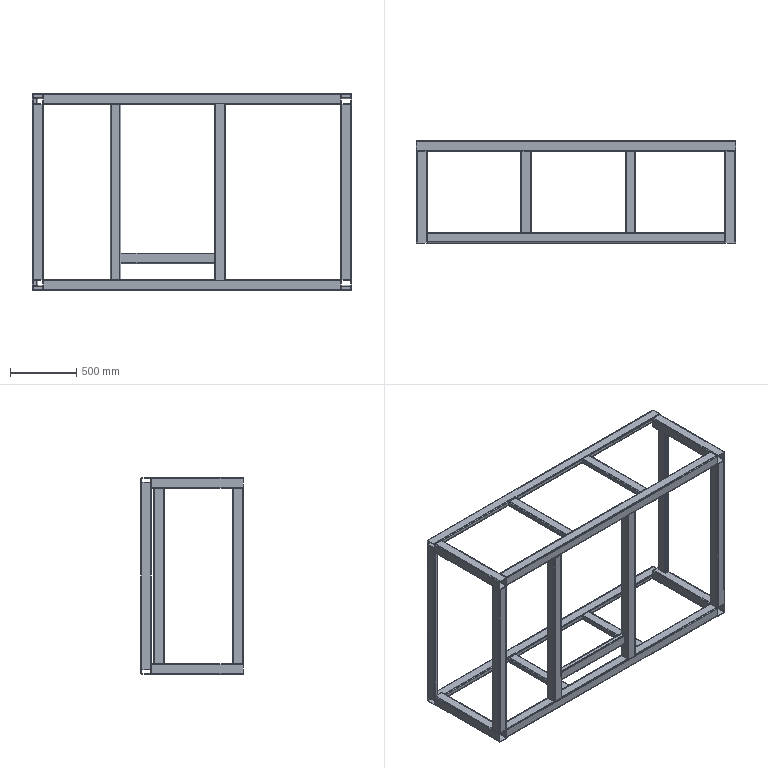Part | SolidWorks | features WeldCornerFeat 5, WeldMemberFeat 4, 3DProfileFeature 2, WeldmentFeature 1 | 19 solids | 342 faces | box 2400 x 770 x 1480 mm | volume 23706901 mm3 | plane 190 | cylinder 152 | commonest cylinder face diameters 8 x72 16 x72 6 x4 12 x4